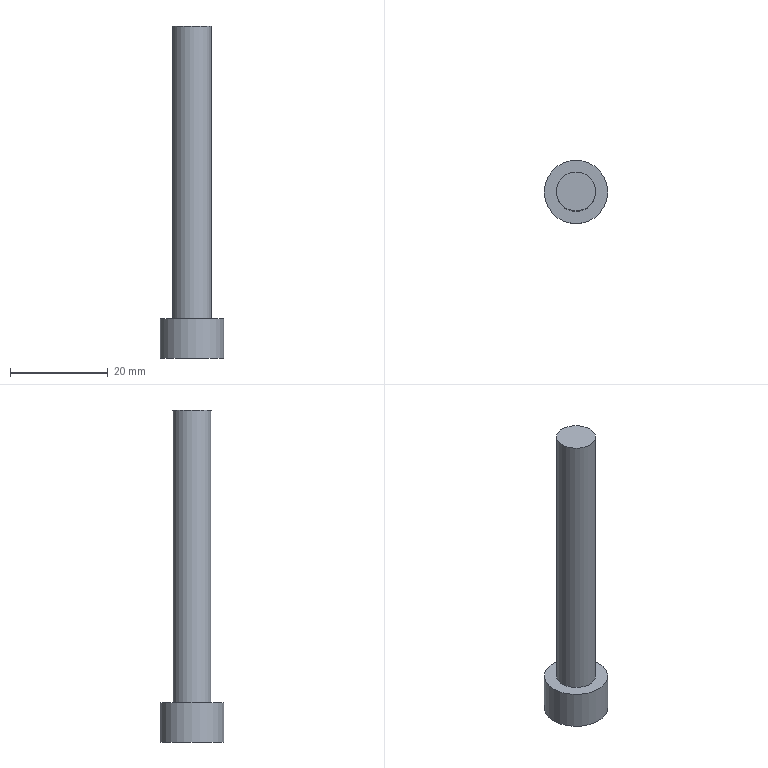Part | STEP file | 1 solid | 12 faces | box 13 x 13 x 68 mm | volume 3913 mm3 | plane 10 | cylinder 2 | commonest cylinder face diameters 8 x1 13 x1
STEP:
#1=CARTESIAN_POINT('',(0.,0.,0.));
#2=DIRECTION('',(0.,0.,1.));
#3=DIRECTION('',(1.,0.,0.));
#4=AXIS2_PLACEMENT_3D('',#1,#2,#3);
#5=CARTESIAN_POINT('',(1550.747,352.48,-93.381));
#6=VERTEX_POINT('',#5);
#7=CARTESIAN_POINT('',(1557.247,352.48,-93.381));
#8=DIRECTION('',(0.,0.,-1.));
#9=DIRECTION('',(-1.,0.,0.));
#10=AXIS2_PLACEMENT_3D('',#7,#8,#9);
#11=CIRCLE('',#10,6.5);
#12=CARTESIAN_POINT('',(1550.747,352.48,-93.381));
#13=DIRECTION('',(0.,0.,1.));
#14=DIRECTION('',(1.,0.,0.));
#15=AXIS2_PLACEMENT_3D('',#12,#13,#14);
#16=PLANE('',#15);
#17=CARTESIAN_POINT('',(0.,0.));
#18=CARTESIAN_POINT('',(0.,11.258));
#19=CARTESIAN_POINT('',(9.75,5.629));
#20=CARTESIAN_POINT('',(19.5,0.));
#21=CARTESIAN_POINT('',(9.75,-5.629));
#22=CARTESIAN_POINT('',(0.,-11.258));
#23=CARTESIAN_POINT('',(0.,0.));
#24=(BOUNDED_CURVE()B_SPLINE_CURVE(2,(#17,#18,#19,#20,#21,#22,#23),.UNSPECIFIED.,.T.,.F.)B_SPLINE_CURVE_WITH_KNOTS((1,2,2,2,2,1),(-2.094,0.,2.094,4.189,6.283,8.378),.UNSPECIFIED.)CURVE()GEOMETRIC_REPRESENTATION_ITEM()RATIONAL_B_SPLINE_CURVE((1.,0.5,1.,0.5,1.,0.5,1.))REPRESENTATION_ITEM(''));
#25=(GEOMETRIC_REPRESENTATION_CONTEXT(2)PARAMETRIC_REPRESENTATION_CONTEXT()REPRESENTATION_CONTEXT('',''));
#26=DEFINITIONAL_REPRESENTATION('',(#24),#25);
#27=PCURVE('',#16,#26);
#28=CARTESIAN_POINT('',(1557.247,352.48,-38.481));
#29=DIRECTION('',(0.,0.,-1.));
#30=DIRECTION('',(-1.,0.,0.));
#31=AXIS2_PLACEMENT_3D('',#28,#29,#30);
#32=CYLINDRICAL_SURFACE('',#31,6.5);
#33=CARTESIAN_POINT('',(0.,54.9));
#34=DIRECTION('',(1.,0.));
#35=VECTOR('',#34,1.);
#36=LINE('',#33,#35);
#37=(GEOMETRIC_REPRESENTATION_CONTEXT(2)PARAMETRIC_REPRESENTATION_CONTEXT()REPRESENTATION_CONTEXT('',''));
#38=DEFINITIONAL_REPRESENTATION('',(#36),#37);
#39=PCURVE('',#32,#38);
#40=SURFACE_CURVE('',#11,(#27,#39),.PCURVE_S1.);
#41=EDGE_CURVE('',#6,#6,#40,.T.);
#42=ORIENTED_EDGE('',*,*,#41,.T.);
#43=EDGE_LOOP('',(#42));
#44=FACE_BOUND('',#43,.T.);
#45=CARTESIAN_POINT('',(1558.979,355.48,-93.381));
#46=VERTEX_POINT('',#45);
#47=CARTESIAN_POINT('',(1555.515,355.48,-93.381));
#48=VERTEX_POINT('',#47);
#49=CARTESIAN_POINT('',(1558.979,355.48,-93.381));
#50=DIRECTION('',(-1.,0.,0.));
#51=VECTOR('',#50,1.);
#52=LINE('',#49,#51);
#53=CARTESIAN_POINT('',(8.232,3.));
#54=DIRECTION('',(-1.,0.));
#55=VECTOR('',#54,1.);
#56=LINE('',#53,#55);
#57=(GEOMETRIC_REPRESENTATION_CONTEXT(2)PARAMETRIC_REPRESENTATION_CONTEXT()REPRESENTATION_CONTEXT('',''));
#58=DEFINITIONAL_REPRESENTATION('',(#56),#57);
#59=PCURVE('',#16,#58);
#60=CARTESIAN_POINT('',(1558.979,355.48,-88.101));
#61=DIRECTION('',(0.,-1.,0.));
#62=DIRECTION('',(-1.,0.,0.));
#63=AXIS2_PLACEMENT_3D('',#60,#61,#62);
#64=PLANE('',#63);
#65=CARTESIAN_POINT('',(0.,5.28));
#66=DIRECTION('',(1.,0.));
#67=VECTOR('',#66,1.);
#68=LINE('',#65,#67);
#69=(GEOMETRIC_REPRESENTATION_CONTEXT(2)PARAMETRIC_REPRESENTATION_CONTEXT()REPRESENTATION_CONTEXT('',''));
#70=DEFINITIONAL_REPRESENTATION('',(#68),#69);
#71=PCURVE('',#64,#70);
#72=SURFACE_CURVE('',#52,(#59,#71),.PCURVE_S1.);
#73=EDGE_CURVE('',#46,#48,#72,.T.);
#74=ORIENTED_EDGE('',*,*,#73,.T.);
#75=CARTESIAN_POINT('',(1553.783,352.48,-93.381));
#76=VERTEX_POINT('',#75);
#77=CARTESIAN_POINT('',(1555.515,355.48,-93.381));
#78=DIRECTION('',(-0.5,-0.866,0.));
#79=VECTOR('',#78,1.);
#80=LINE('',#77,#79);
#81=CARTESIAN_POINT('',(4.768,3.));
#82=DIRECTION('',(-0.5,-0.866));
#83=VECTOR('',#82,1.);
#84=LINE('',#81,#83);
#85=(GEOMETRIC_REPRESENTATION_CONTEXT(2)PARAMETRIC_REPRESENTATION_CONTEXT()REPRESENTATION_CONTEXT('',''));
#86=DEFINITIONAL_REPRESENTATION('',(#84),#85);
#87=PCURVE('',#16,#86);
#88=CARTESIAN_POINT('',(1555.515,355.48,-88.101));
#89=DIRECTION('',(0.866,-0.5,0.));
#90=DIRECTION('',(-0.5,-0.866,0.));
#91=AXIS2_PLACEMENT_3D('',#88,#89,#90);
#92=PLANE('',#91);
#93=CARTESIAN_POINT('',(0.,5.28));
#94=DIRECTION('',(1.,0.));
#95=VECTOR('',#94,1.);
#96=LINE('',#93,#95);
#97=(GEOMETRIC_REPRESENTATION_CONTEXT(2)PARAMETRIC_REPRESENTATION_CONTEXT()REPRESENTATION_CONTEXT('',''));
#98=DEFINITIONAL_REPRESENTATION('',(#96),#97);
#99=PCURVE('',#92,#98);
#100=SURFACE_CURVE('',#80,(#87,#99),.PCURVE_S1.);
#101=EDGE_CURVE('',#48,#76,#100,.T.);
#102=ORIENTED_EDGE('',*,*,#101,.T.);
#103=CARTESIAN_POINT('',(1555.515,349.48,-93.381));
#104=VERTEX_POINT('',#103);
#105=CARTESIAN_POINT('',(1553.783,352.48,-93.381));
#106=DIRECTION('',(0.5,-0.866,0.));
#107=VECTOR('',#106,1.);
#108=LINE('',#105,#107);
#109=CARTESIAN_POINT('',(3.036,0.));
#110=DIRECTION('',(0.5,-0.866));
#111=VECTOR('',#110,1.);
#112=LINE('',#109,#111);
#113=(GEOMETRIC_REPRESENTATION_CONTEXT(2)PARAMETRIC_REPRESENTATION_CONTEXT()REPRESENTATION_CONTEXT('',''));
#114=DEFINITIONAL_REPRESENTATION('',(#112),#113);
#115=PCURVE('',#16,#114);
#116=CARTESIAN_POINT('',(1553.783,352.48,-88.101));
#117=DIRECTION('',(0.866,0.5,0.));
#118=DIRECTION('',(0.5,-0.866,0.));
#119=AXIS2_PLACEMENT_3D('',#116,#117,#118);
#120=PLANE('',#119);
#121=CARTESIAN_POINT('',(0.,5.28));
#122=DIRECTION('',(1.,0.));
#123=VECTOR('',#122,1.);
#124=LINE('',#121,#123);
#125=(GEOMETRIC_REPRESENTATION_CONTEXT(2)PARAMETRIC_REPRESENTATION_CONTEXT()REPRESENTATION_CONTEXT('',''));
#126=DEFINITIONAL_REPRESENTATION('',(#124),#125);
#127=PCURVE('',#120,#126);
#128=SURFACE_CURVE('',#108,(#115,#127),.PCURVE_S1.);
#129=EDGE_CURVE('',#76,#104,#128,.T.);
#130=ORIENTED_EDGE('',*,*,#129,.T.);
#131=CARTESIAN_POINT('',(1558.979,349.48,-93.381));
#132=VERTEX_POINT('',#131);
#133=CARTESIAN_POINT('',(1555.515,349.48,-93.381));
#134=DIRECTION('',(1.,0.,0.));
#135=VECTOR('',#134,1.);
#136=LINE('',#133,#135);
#137=CARTESIAN_POINT('',(4.768,-3.));
#138=DIRECTION('',(1.,0.));
#139=VECTOR('',#138,1.);
#140=LINE('',#137,#139);
#141=(GEOMETRIC_REPRESENTATION_CONTEXT(2)PARAMETRIC_REPRESENTATION_CONTEXT()REPRESENTATION_CONTEXT('',''));
#142=DEFINITIONAL_REPRESENTATION('',(#140),#141);
#143=PCURVE('',#16,#142);
#144=CARTESIAN_POINT('',(1555.515,349.48,-88.101));
#145=DIRECTION('',(0.,1.,0.));
#146=DIRECTION('',(1.,0.,0.));
#147=AXIS2_PLACEMENT_3D('',#144,#145,#146);
#148=PLANE('',#147);
#149=CARTESIAN_POINT('',(0.,5.28));
#150=DIRECTION('',(1.,0.));
#151=VECTOR('',#150,1.);
#152=LINE('',#149,#151);
#153=(GEOMETRIC_REPRESENTATION_CONTEXT(2)PARAMETRIC_REPRESENTATION_CONTEXT()REPRESENTATION_CONTEXT('',''));
#154=DEFINITIONAL_REPRESENTATION('',(#152),#153);
#155=PCURVE('',#148,#154);
#156=SURFACE_CURVE('',#136,(#143,#155),.PCURVE_S1.);
#157=EDGE_CURVE('',#104,#132,#156,.T.);
#158=ORIENTED_EDGE('',*,*,#157,.T.);
#159=CARTESIAN_POINT('',(1560.711,352.48,-93.381));
#160=VERTEX_POINT('',#159);
#161=CARTESIAN_POINT('',(1558.979,349.48,-93.381));
#162=DIRECTION('',(0.5,0.866,0.));
#163=VECTOR('',#162,1.);
#164=LINE('',#161,#163);
#165=CARTESIAN_POINT('',(8.232,-3.));
#166=DIRECTION('',(0.5,0.866));
#167=VECTOR('',#166,1.);
#168=LINE('',#165,#167);
#169=(GEOMETRIC_REPRESENTATION_CONTEXT(2)PARAMETRIC_REPRESENTATION_CONTEXT()REPRESENTATION_CONTEXT('',''));
#170=DEFINITIONAL_REPRESENTATION('',(#168),#169);
#171=PCURVE('',#16,#170);
#172=CARTESIAN_POINT('',(1558.979,349.48,-88.101));
#173=DIRECTION('',(-0.866,0.5,0.));
#174=DIRECTION('',(0.5,0.866,0.));
#175=AXIS2_PLACEMENT_3D('',#172,#173,#174);
#176=PLANE('',#175);
#177=CARTESIAN_POINT('',(0.,5.28));
#178=DIRECTION('',(1.,0.));
#179=VECTOR('',#178,1.);
#180=LINE('',#177,#179);
#181=(GEOMETRIC_REPRESENTATION_CONTEXT(2)PARAMETRIC_REPRESENTATION_CONTEXT()REPRESENTATION_CONTEXT('',''));
#182=DEFINITIONAL_REPRESENTATION('',(#180),#181);
#183=PCURVE('',#176,#182);
#184=SURFACE_CURVE('',#164,(#171,#183),.PCURVE_S1.);
#185=EDGE_CURVE('',#132,#160,#184,.T.);
#186=ORIENTED_EDGE('',*,*,#185,.T.);
#187=CARTESIAN_POINT('',(1560.711,352.48,-93.381));
#188=DIRECTION('',(-0.5,0.866,0.));
#189=VECTOR('',#188,1.);
#190=LINE('',#187,#189);
#191=CARTESIAN_POINT('',(9.964,0.));
#192=DIRECTION('',(-0.5,0.866));
#193=VECTOR('',#192,1.);
#194=LINE('',#191,#193);
#195=(GEOMETRIC_REPRESENTATION_CONTEXT(2)PARAMETRIC_REPRESENTATION_CONTEXT()REPRESENTATION_CONTEXT('',''));
#196=DEFINITIONAL_REPRESENTATION('',(#194),#195);
#197=PCURVE('',#16,#196);
#198=CARTESIAN_POINT('',(1560.711,352.48,-88.101));
#199=DIRECTION('',(-0.866,-0.5,0.));
#200=DIRECTION('',(-0.5,0.866,0.));
#201=AXIS2_PLACEMENT_3D('',#198,#199,#200);
#202=PLANE('',#201);
#203=CARTESIAN_POINT('',(0.,5.28));
#204=DIRECTION('',(1.,0.));
#205=VECTOR('',#204,1.);
#206=LINE('',#203,#205);
#207=(GEOMETRIC_REPRESENTATION_CONTEXT(2)PARAMETRIC_REPRESENTATION_CONTEXT()REPRESENTATION_CONTEXT('',''));
#208=DEFINITIONAL_REPRESENTATION('',(#206),#207);
#209=PCURVE('',#202,#208);
#210=SURFACE_CURVE('',#190,(#197,#209),.PCURVE_S1.);
#211=EDGE_CURVE('',#160,#46,#210,.T.);
#212=ORIENTED_EDGE('',*,*,#211,.T.);
#213=EDGE_LOOP('',(#74,#102,#130,#158,#186,#212));
#214=FACE_BOUND('',#213,.T.);
#215=ADVANCED_FACE('',(#44,#214),#16,.F.);
#216=ORIENTED_EDGE('',*,*,#41,.F.);
#217=CARTESIAN_POINT('',(1550.747,352.48,-85.381));
#218=VERTEX_POINT('',#217);
#219=CARTESIAN_POINT('',(1550.747,352.48,-85.381));
#220=CARTESIAN_POINT('',(1550.747,352.48,-93.381));
#221=B_SPLINE_CURVE_WITH_KNOTS('',1,(#219,#220),.UNSPECIFIED.,.F.,.F.,(2,2),(46.9,54.9),.PIECEWISE_BEZIER_KNOTS.);
#222=CARTESIAN_POINT('',(0.,0.));
#223=DIRECTION('',(0.,1.));
#224=VECTOR('',#223,1.);
#225=LINE('',#222,#224);
#226=(GEOMETRIC_REPRESENTATION_CONTEXT(2)PARAMETRIC_REPRESENTATION_CONTEXT()REPRESENTATION_CONTEXT('',''));
#227=DEFINITIONAL_REPRESENTATION('',(#225),#226);
#228=PCURVE('',#32,#227);
#229=CARTESIAN_POINT('',(6.283,0.));
#230=DIRECTION('',(0.,1.));
#231=VECTOR('',#230,1.);
#232=LINE('',#229,#231);
#233=(GEOMETRIC_REPRESENTATION_CONTEXT(2)PARAMETRIC_REPRESENTATION_CONTEXT()REPRESENTATION_CONTEXT('',''));
#234=DEFINITIONAL_REPRESENTATION('',(#232),#233);
#235=PCURVE('',#32,#234);
#236=SEAM_CURVE('',#221,(#228,#235),.PCURVE_S1.);
#237=EDGE_CURVE('',#218,#6,#236,.T.);
#238=ORIENTED_EDGE('',*,*,#237,.F.);
#239=CARTESIAN_POINT('',(1557.247,352.48,-85.381));
#240=DIRECTION('',(0.,0.,-1.));
#241=DIRECTION('',(-1.,0.,0.));
#242=AXIS2_PLACEMENT_3D('',#239,#240,#241);
#243=CIRCLE('',#242,6.5);
#244=CARTESIAN_POINT('',(0.,46.9));
#245=DIRECTION('',(1.,0.));
#246=VECTOR('',#245,1.);
#247=LINE('',#244,#246);
#248=(GEOMETRIC_REPRESENTATION_CONTEXT(2)PARAMETRIC_REPRESENTATION_CONTEXT()REPRESENTATION_CONTEXT('',''));
#249=DEFINITIONAL_REPRESENTATION('',(#247),#248);
#250=PCURVE('',#32,#249);
#251=CARTESIAN_POINT('',(1553.247,352.48,-85.381));
#252=DIRECTION('',(0.,0.,-1.));
#253=DIRECTION('',(-1.,0.,0.));
#254=AXIS2_PLACEMENT_3D('',#251,#252,#253);
#255=PLANE('',#254);
#256=CARTESIAN_POINT('',(-4.,0.));
#257=DIRECTION('',(1.,0.));
#258=AXIS2_PLACEMENT_2D('',#256,#257);
#259=CIRCLE('',#258,6.5);
#260=(GEOMETRIC_REPRESENTATION_CONTEXT(2)PARAMETRIC_REPRESENTATION_CONTEXT()REPRESENTATION_CONTEXT('',''));
#261=DEFINITIONAL_REPRESENTATION('',(#259),#260);
#262=PCURVE('',#255,#261);
#263=SURFACE_CURVE('',#243,(#250,#262),.PCURVE_S1.);
#264=EDGE_CURVE('',#218,#218,#263,.T.);
#265=ORIENTED_EDGE('',*,*,#264,.T.);
#266=ORIENTED_EDGE('',*,*,#237,.T.);
#267=EDGE_LOOP('',(#216,#238,#265,#266));
#268=FACE_BOUND('',#267,.T.);
#269=ADVANCED_FACE('',(#268),#32,.T.);
#270=ORIENTED_EDGE('',*,*,#264,.F.);
#271=EDGE_LOOP('',(#270));
#272=FACE_BOUND('',#271,.T.);
#273=CARTESIAN_POINT('',(1553.247,352.48,-85.381));
#274=VERTEX_POINT('',#273);
#275=CARTESIAN_POINT('',(1557.247,352.48,-85.381));
#276=DIRECTION('',(0.,0.,-1.));
#277=DIRECTION('',(-1.,0.,0.));
#278=AXIS2_PLACEMENT_3D('',#275,#276,#277);
#279=CIRCLE('',#278,4.);
#280=CARTESIAN_POINT('',(-4.,0.));
#281=DIRECTION('',(1.,0.));
#282=AXIS2_PLACEMENT_2D('',#280,#281);
#283=CIRCLE('',#282,4.);
#284=(GEOMETRIC_REPRESENTATION_CONTEXT(2)PARAMETRIC_REPRESENTATION_CONTEXT()REPRESENTATION_CONTEXT('',''));
#285=DEFINITIONAL_REPRESENTATION('',(#283),#284);
#286=PCURVE('',#255,#285);
#287=CARTESIAN_POINT('',(1557.247,352.48,-38.481));
#288=DIRECTION('',(0.,0.,-1.));
#289=DIRECTION('',(-1.,0.,0.));
#290=AXIS2_PLACEMENT_3D('',#287,#288,#289);
#291=CYLINDRICAL_SURFACE('',#290,4.);
#292=CARTESIAN_POINT('',(0.,46.9));
#293=DIRECTION('',(1.,0.));
#294=VECTOR('',#293,1.);
#295=LINE('',#292,#294);
#296=(GEOMETRIC_REPRESENTATION_CONTEXT(2)PARAMETRIC_REPRESENTATION_CONTEXT()REPRESENTATION_CONTEXT('',''));
#297=DEFINITIONAL_REPRESENTATION('',(#295),#296);
#298=PCURVE('',#291,#297);
#299=SURFACE_CURVE('',#279,(#286,#298),.PCURVE_S1.);
#300=EDGE_CURVE('',#274,#274,#299,.T.);
#301=ORIENTED_EDGE('',*,*,#300,.T.);
#302=EDGE_LOOP('',(#301));
#303=FACE_BOUND('',#302,.T.);
#304=ADVANCED_FACE('',(#272,#303),#255,.F.);
#305=ORIENTED_EDGE('',*,*,#300,.F.);
#306=CARTESIAN_POINT('',(1553.247,352.48,-25.381));
#307=VERTEX_POINT('',#306);
#308=CARTESIAN_POINT('',(1553.247,352.48,-25.381));
#309=CARTESIAN_POINT('',(1553.247,352.48,-85.381));
#310=B_SPLINE_CURVE_WITH_KNOTS('',1,(#308,#309),.UNSPECIFIED.,.F.,.F.,(2,2),(-13.1,46.9),.PIECEWISE_BEZIER_KNOTS.);
#311=CARTESIAN_POINT('',(0.,0.));
#312=DIRECTION('',(0.,1.));
#313=VECTOR('',#312,1.);
#314=LINE('',#311,#313);
#315=(GEOMETRIC_REPRESENTATION_CONTEXT(2)PARAMETRIC_REPRESENTATION_CONTEXT()REPRESENTATION_CONTEXT('',''));
#316=DEFINITIONAL_REPRESENTATION('',(#314),#315);
#317=PCURVE('',#291,#316);
#318=CARTESIAN_POINT('',(6.283,0.));
#319=DIRECTION('',(0.,1.));
#320=VECTOR('',#319,1.);
#321=LINE('',#318,#320);
#322=(GEOMETRIC_REPRESENTATION_CONTEXT(2)PARAMETRIC_REPRESENTATION_CONTEXT()REPRESENTATION_CONTEXT('',''));
#323=DEFINITIONAL_REPRESENTATION('',(#321),#322);
#324=PCURVE('',#291,#323);
#325=SEAM_CURVE('',#310,(#317,#324),.PCURVE_S1.);
#326=EDGE_CURVE('',#307,#274,#325,.T.);
#327=ORIENTED_EDGE('',*,*,#326,.F.);
#328=CARTESIAN_POINT('',(1557.247,352.48,-25.381));
#329=DIRECTION('',(0.,0.,-1.));
#330=DIRECTION('',(-1.,0.,0.));
#331=AXIS2_PLACEMENT_3D('',#328,#329,#330);
#332=CIRCLE('',#331,4.);
#333=CARTESIAN_POINT('',(0.,-13.1));
#334=DIRECTION('',(1.,0.));
#335=VECTOR('',#334,1.);
#336=LINE('',#333,#335);
#337=(GEOMETRIC_REPRESENTATION_CONTEXT(2)PARAMETRIC_REPRESENTATION_CONTEXT()REPRESENTATION_CONTEXT('',''));
#338=DEFINITIONAL_REPRESENTATION('',(#336),#337);
#339=PCURVE('',#291,#338);
#340=CARTESIAN_POINT('',(1557.247,352.48,-25.381));
#341=DIRECTION('',(0.,0.,-1.));
#342=DIRECTION('',(-1.,0.,0.));
#343=AXIS2_PLACEMENT_3D('',#340,#341,#342);
#344=PLANE('',#343);
#345=CARTESIAN_POINT('',(0.,0.));
#346=DIRECTION('',(1.,0.));
#347=AXIS2_PLACEMENT_2D('',#345,#346);
#348=CIRCLE('',#347,4.);
#349=(GEOMETRIC_REPRESENTATION_CONTEXT(2)PARAMETRIC_REPRESENTATION_CONTEXT()REPRESENTATION_CONTEXT('',''));
#350=DEFINITIONAL_REPRESENTATION('',(#348),#349);
#351=PCURVE('',#344,#350);
#352=SURFACE_CURVE('',#332,(#339,#351),.PCURVE_S1.);
#353=EDGE_CURVE('',#307,#307,#352,.T.);
#354=ORIENTED_EDGE('',*,*,#353,.T.);
#355=ORIENTED_EDGE('',*,*,#326,.T.);
#356=EDGE_LOOP('',(#305,#327,#354,#355));
#357=FACE_BOUND('',#356,.T.);
#358=ADVANCED_FACE('',(#357),#291,.T.);
#359=ORIENTED_EDGE('',*,*,#353,.F.);
#360=EDGE_LOOP('',(#359));
#361=FACE_BOUND('',#360,.T.);
#362=ADVANCED_FACE('',(#361),#344,.F.);
#363=ORIENTED_EDGE('',*,*,#73,.F.);
#364=CARTESIAN_POINT('',(1558.979,355.48,-88.101));
#365=VERTEX_POINT('',#364);
#366=CARTESIAN_POINT('',(1558.979,355.48,-88.101));
#367=DIRECTION('',(0.,0.,1.));
#368=VECTOR('',#367,1.);
#369=LINE('',#366,#368);
#370=CARTESIAN_POINT('',(0.,0.));
#371=DIRECTION('',(0.,-1.));
#372=VECTOR('',#371,1.);
#373=LINE('',#370,#372);
#374=(GEOMETRIC_REPRESENTATION_CONTEXT(2)PARAMETRIC_REPRESENTATION_CONTEXT()REPRESENTATION_CONTEXT('',''));
#375=DEFINITIONAL_REPRESENTATION('',(#373),#374);
#376=PCURVE('',#64,#375);
#377=CARTESIAN_POINT('',(3.464,0.));
#378=DIRECTION('',(0.,-1.));
#379=VECTOR('',#378,1.);
#380=LINE('',#377,#379);
#381=(GEOMETRIC_REPRESENTATION_CONTEXT(2)PARAMETRIC_REPRESENTATION_CONTEXT()REPRESENTATION_CONTEXT('',''));
#382=DEFINITIONAL_REPRESENTATION('',(#380),#381);
#383=PCURVE('',#202,#382);
#384=SURFACE_CURVE('',#369,(#376,#383),.PCURVE_S1.);
#385=EDGE_CURVE('',#46,#365,#384,.T.);
#386=ORIENTED_EDGE('',*,*,#385,.T.);
#387=CARTESIAN_POINT('',(1555.515,355.48,-88.101));
#388=VERTEX_POINT('',#387);
#389=CARTESIAN_POINT('',(1558.979,355.48,-88.101));
#390=DIRECTION('',(1.,0.,0.));
#391=VECTOR('',#390,1.);
#392=LINE('',#389,#391);
#393=CARTESIAN_POINT('',(0.,0.));
#394=DIRECTION('',(-1.,0.));
#395=VECTOR('',#394,1.);
#396=LINE('',#393,#395);
#397=(GEOMETRIC_REPRESENTATION_CONTEXT(2)PARAMETRIC_REPRESENTATION_CONTEXT()REPRESENTATION_CONTEXT('',''));
#398=DEFINITIONAL_REPRESENTATION('',(#396),#397);
#399=PCURVE('',#64,#398);
#400=CARTESIAN_POINT('',(1557.247,352.48,-88.101));
#401=DIRECTION('',(0.,0.,1.));
#402=DIRECTION('',(1.,0.,0.));
#403=AXIS2_PLACEMENT_3D('',#400,#401,#402);
#404=PLANE('',#403);
#405=CARTESIAN_POINT('',(1.732,3.));
#406=DIRECTION('',(1.,0.));
#407=VECTOR('',#406,1.);
#408=LINE('',#405,#407);
#409=(GEOMETRIC_REPRESENTATION_CONTEXT(2)PARAMETRIC_REPRESENTATION_CONTEXT()REPRESENTATION_CONTEXT('',''));
#410=DEFINITIONAL_REPRESENTATION('',(#408),#409);
#411=PCURVE('',#404,#410);
#412=SURFACE_CURVE('',#392,(#399,#411),.PCURVE_S1.);
#413=EDGE_CURVE('',#388,#365,#412,.T.);
#414=ORIENTED_EDGE('',*,*,#413,.F.);
#415=CARTESIAN_POINT('',(1555.515,355.48,-88.101));
#416=DIRECTION('',(0.,0.,1.));
#417=VECTOR('',#416,1.);
#418=LINE('',#415,#417);
#419=CARTESIAN_POINT('',(3.464,0.));
#420=DIRECTION('',(0.,-1.));
#421=VECTOR('',#420,1.);
#422=LINE('',#419,#421);
#423=(GEOMETRIC_REPRESENTATION_CONTEXT(2)PARAMETRIC_REPRESENTATION_CONTEXT()REPRESENTATION_CONTEXT('',''));
#424=DEFINITIONAL_REPRESENTATION('',(#422),#423);
#425=PCURVE('',#64,#424);
#426=CARTESIAN_POINT('',(0.,0.));
#427=DIRECTION('',(0.,-1.));
#428=VECTOR('',#427,1.);
#429=LINE('',#426,#428);
#430=(GEOMETRIC_REPRESENTATION_CONTEXT(2)PARAMETRIC_REPRESENTATION_CONTEXT()REPRESENTATION_CONTEXT('',''));
#431=DEFINITIONAL_REPRESENTATION('',(#429),#430);
#432=PCURVE('',#92,#431);
#433=SURFACE_CURVE('',#418,(#425,#432),.PCURVE_S1.);
#434=EDGE_CURVE('',#48,#388,#433,.T.);
#435=ORIENTED_EDGE('',*,*,#434,.F.);
#436=EDGE_LOOP('',(#363,#386,#414,#435));
#437=FACE_BOUND('',#436,.T.);
#438=ADVANCED_FACE('',(#437),#64,.T.);
#439=ORIENTED_EDGE('',*,*,#101,.F.);
#440=ORIENTED_EDGE('',*,*,#434,.T.);
#441=CARTESIAN_POINT('',(1553.783,352.48,-88.101));
#442=VERTEX_POINT('',#441);
#443=CARTESIAN_POINT('',(1555.515,355.48,-88.101));
#444=DIRECTION('',(0.5,0.866,0.));
#445=VECTOR('',#444,1.);
#446=LINE('',#443,#445);
#447=CARTESIAN_POINT('',(0.,0.));
#448=DIRECTION('',(-1.,0.));
#449=VECTOR('',#448,1.);
#450=LINE('',#447,#449);
#451=(GEOMETRIC_REPRESENTATION_CONTEXT(2)PARAMETRIC_REPRESENTATION_CONTEXT()REPRESENTATION_CONTEXT('',''));
#452=DEFINITIONAL_REPRESENTATION('',(#450),#451);
#453=PCURVE('',#92,#452);
#454=CARTESIAN_POINT('',(-1.732,3.));
#455=DIRECTION('',(0.5,0.866));
#456=VECTOR('',#455,1.);
#457=LINE('',#454,#456);
#458=(GEOMETRIC_REPRESENTATION_CONTEXT(2)PARAMETRIC_REPRESENTATION_CONTEXT()REPRESENTATION_CONTEXT('',''));
#459=DEFINITIONAL_REPRESENTATION('',(#457),#458);
#460=PCURVE('',#404,#459);
#461=SURFACE_CURVE('',#446,(#453,#460),.PCURVE_S1.);
#462=EDGE_CURVE('',#442,#388,#461,.T.);
#463=ORIENTED_EDGE('',*,*,#462,.F.);
#464=CARTESIAN_POINT('',(1553.783,352.48,-88.101));
#465=DIRECTION('',(0.,0.,1.));
#466=VECTOR('',#465,1.);
#467=LINE('',#464,#466);
#468=CARTESIAN_POINT('',(3.464,0.));
#469=DIRECTION('',(0.,-1.));
#470=VECTOR('',#469,1.);
#471=LINE('',#468,#470);
#472=(GEOMETRIC_REPRESENTATION_CONTEXT(2)PARAMETRIC_REPRESENTATION_CONTEXT()REPRESENTATION_CONTEXT('',''));
#473=DEFINITIONAL_REPRESENTATION('',(#471),#472);
#474=PCURVE('',#92,#473);
#475=CARTESIAN_POINT('',(0.,0.));
#476=DIRECTION('',(0.,-1.));
#477=VECTOR('',#476,1.);
#478=LINE('',#475,#477);
#479=(GEOMETRIC_REPRESENTATION_CONTEXT(2)PARAMETRIC_REPRESENTATION_CONTEXT()REPRESENTATION_CONTEXT('',''));
#480=DEFINITIONAL_REPRESENTATION('',(#478),#479);
#481=PCURVE('',#120,#480);
#482=SURFACE_CURVE('',#467,(#474,#481),.PCURVE_S1.);
#483=EDGE_CURVE('',#76,#442,#482,.T.);
#484=ORIENTED_EDGE('',*,*,#483,.F.);
#485=EDGE_LOOP('',(#439,#440,#463,#484));
#486=FACE_BOUND('',#485,.T.);
#487=ADVANCED_FACE('',(#486),#92,.T.);
#488=ORIENTED_EDGE('',*,*,#129,.F.);
#489=ORIENTED_EDGE('',*,*,#483,.T.);
#490=CARTESIAN_POINT('',(1555.515,349.48,-88.101));
#491=VERTEX_POINT('',#490);
#492=CARTESIAN_POINT('',(1553.783,352.48,-88.101));
#493=DIRECTION('',(-0.5,0.866,0.));
#494=VECTOR('',#493,1.);
#495=LINE('',#492,#494);
#496=CARTESIAN_POINT('',(0.,0.));
#497=DIRECTION('',(-1.,0.));
#498=VECTOR('',#497,1.);
#499=LINE('',#496,#498);
#500=(GEOMETRIC_REPRESENTATION_CONTEXT(2)PARAMETRIC_REPRESENTATION_CONTEXT()REPRESENTATION_CONTEXT('',''));
#501=DEFINITIONAL_REPRESENTATION('',(#499),#500);
#502=PCURVE('',#120,#501);
#503=CARTESIAN_POINT('',(-3.464,0.));
#504=DIRECTION('',(-0.5,0.866));
#505=VECTOR('',#504,1.);
#506=LINE('',#503,#505);
#507=(GEOMETRIC_REPRESENTATION_CONTEXT(2)PARAMETRIC_REPRESENTATION_CONTEXT()REPRESENTATION_CONTEXT('',''));
#508=DEFINITIONAL_REPRESENTATION('',(#506),#507);
#509=PCURVE('',#404,#508);
#510=SURFACE_CURVE('',#495,(#502,#509),.PCURVE_S1.);
#511=EDGE_CURVE('',#491,#442,#510,.T.);
#512=ORIENTED_EDGE('',*,*,#511,.F.);
#513=CARTESIAN_POINT('',(1555.515,349.48,-88.101));
#514=DIRECTION('',(0.,0.,1.));
#515=VECTOR('',#514,1.);
#516=LINE('',#513,#515);
#517=CARTESIAN_POINT('',(3.464,0.));
#518=DIRECTION('',(0.,-1.));
#519=VECTOR('',#518,1.);
#520=LINE('',#517,#519);
#521=(GEOMETRIC_REPRESENTATION_CONTEXT(2)PARAMETRIC_REPRESENTATION_CONTEXT()REPRESENTATION_CONTEXT('',''));
#522=DEFINITIONAL_REPRESENTATION('',(#520),#521);
#523=PCURVE('',#120,#522);
#524=CARTESIAN_POINT('',(0.,0.));
#525=DIRECTION('',(0.,-1.));
#526=VECTOR('',#525,1.);
#527=LINE('',#524,#526);
#528=(GEOMETRIC_REPRESENTATION_CONTEXT(2)PARAMETRIC_REPRESENTATION_CONTEXT()REPRESENTATION_CONTEXT('',''));
#529=DEFINITIONAL_REPRESENTATION('',(#527),#528);
#530=PCURVE('',#148,#529);
#531=SURFACE_CURVE('',#516,(#523,#530),.PCURVE_S1.);
#532=EDGE_CURVE('',#104,#491,#531,.T.);
#533=ORIENTED_EDGE('',*,*,#532,.F.);
#534=EDGE_LOOP('',(#488,#489,#512,#533));
#535=FACE_BOUND('',#534,.T.);
#536=ADVANCED_FACE('',(#535),#120,.T.);
#537=ORIENTED_EDGE('',*,*,#157,.F.);
#538=ORIENTED_EDGE('',*,*,#532,.T.);
#539=CARTESIAN_POINT('',(1558.979,349.48,-88.101));
#540=VERTEX_POINT('',#539);
#541=CARTESIAN_POINT('',(1555.515,349.48,-88.101));
#542=DIRECTION('',(-1.,0.,0.));
#543=VECTOR('',#542,1.);
#544=LINE('',#541,#543);
#545=CARTESIAN_POINT('',(0.,0.));
#546=DIRECTION('',(-1.,0.));
#547=VECTOR('',#546,1.);
#548=LINE('',#545,#547);
#549=(GEOMETRIC_REPRESENTATION_CONTEXT(2)PARAMETRIC_REPRESENTATION_CONTEXT()REPRESENTATION_CONTEXT('',''));
#550=DEFINITIONAL_REPRESENTATION('',(#548),#549);
#551=PCURVE('',#148,#550);
#552=CARTESIAN_POINT('',(-1.732,-3.));
#553=DIRECTION('',(-1.,0.));
#554=VECTOR('',#553,1.);
#555=LINE('',#552,#554);
#556=(GEOMETRIC_REPRESENTATION_CONTEXT(2)PARAMETRIC_REPRESENTATION_CONTEXT()REPRESENTATION_CONTEXT('',''));
#557=DEFINITIONAL_REPRESENTATION('',(#555),#556);
#558=PCURVE('',#404,#557);
#559=SURFACE_CURVE('',#544,(#551,#558),.PCURVE_S1.);
#560=EDGE_CURVE('',#540,#491,#559,.T.);
#561=ORIENTED_EDGE('',*,*,#560,.F.);
#562=CARTESIAN_POINT('',(1558.979,349.48,-88.101));
#563=DIRECTION('',(0.,0.,1.));
#564=VECTOR('',#563,1.);
#565=LINE('',#562,#564);
#566=CARTESIAN_POINT('',(3.464,0.));
#567=DIRECTION('',(0.,-1.));
#568=VECTOR('',#567,1.);
#569=LINE('',#566,#568);
#570=(GEOMETRIC_REPRESENTATION_CONTEXT(2)PARAMETRIC_REPRESENTATION_CONTEXT()REPRESENTATION_CONTEXT('',''));
#571=DEFINITIONAL_REPRESENTATION('',(#569),#570);
#572=PCURVE('',#148,#571);
#573=CARTESIAN_POINT('',(0.,0.));
#574=DIRECTION('',(0.,-1.));
#575=VECTOR('',#574,1.);
#576=LINE('',#573,#575);
#577=(GEOMETRIC_REPRESENTATION_CONTEXT(2)PARAMETRIC_REPRESENTATION_CONTEXT()REPRESENTATION_CONTEXT('',''));
#578=DEFINITIONAL_REPRESENTATION('',(#576),#577);
#579=PCURVE('',#176,#578);
#580=SURFACE_CURVE('',#565,(#572,#579),.PCURVE_S1.);
#581=EDGE_CURVE('',#132,#540,#580,.T.);
#582=ORIENTED_EDGE('',*,*,#581,.F.);
#583=EDGE_LOOP('',(#537,#538,#561,#582));
#584=FACE_BOUND('',#583,.T.);
#585=ADVANCED_FACE('',(#584),#148,.T.);
#586=ORIENTED_EDGE('',*,*,#185,.F.);
#587=ORIENTED_EDGE('',*,*,#581,.T.);
#588=CARTESIAN_POINT('',(1560.711,352.48,-88.101));
#589=VERTEX_POINT('',#588);
#590=CARTESIAN_POINT('',(1558.979,349.48,-88.101));
#591=DIRECTION('',(-0.5,-0.866,0.));
#592=VECTOR('',#591,1.);
#593=LINE('',#590,#592);
#594=CARTESIAN_POINT('',(0.,0.));
#595=DIRECTION('',(-1.,0.));
#596=VECTOR('',#595,1.);
#597=LINE('',#594,#596);
#598=(GEOMETRIC_REPRESENTATION_CONTEXT(2)PARAMETRIC_REPRESENTATION_CONTEXT()REPRESENTATION_CONTEXT('',''));
#599=DEFINITIONAL_REPRESENTATION('',(#597),#598);
#600=PCURVE('',#176,#599);
#601=CARTESIAN_POINT('',(1.732,-3.));
#602=DIRECTION('',(-0.5,-0.866));
#603=VECTOR('',#602,1.);
#604=LINE('',#601,#603);
#605=(GEOMETRIC_REPRESENTATION_CONTEXT(2)PARAMETRIC_REPRESENTATION_CONTEXT()REPRESENTATION_CONTEXT('',''));
#606=DEFINITIONAL_REPRESENTATION('',(#604),#605);
#607=PCURVE('',#404,#606);
#608=SURFACE_CURVE('',#593,(#600,#607),.PCURVE_S1.);
#609=EDGE_CURVE('',#589,#540,#608,.T.);
#610=ORIENTED_EDGE('',*,*,#609,.F.);
#611=CARTESIAN_POINT('',(1560.711,352.48,-88.101));
#612=DIRECTION('',(0.,0.,1.));
#613=VECTOR('',#612,1.);
#614=LINE('',#611,#613);
#615=CARTESIAN_POINT('',(3.464,0.));
#616=DIRECTION('',(0.,-1.));
#617=VECTOR('',#616,1.);
#618=LINE('',#615,#617);
#619=(GEOMETRIC_REPRESENTATION_CONTEXT(2)PARAMETRIC_REPRESENTATION_CONTEXT()REPRESENTATION_CONTEXT('',''));
#620=DEFINITIONAL_REPRESENTATION('',(#618),#619);
#621=PCURVE('',#176,#620);
#622=CARTESIAN_POINT('',(0.,0.));
#623=DIRECTION('',(0.,-1.));
#624=VECTOR('',#623,1.);
#625=LINE('',#622,#624);
#626=(GEOMETRIC_REPRESENTATION_CONTEXT(2)PARAMETRIC_REPRESENTATION_CONTEXT()REPRESENTATION_CONTEXT('',''));
#627=DEFINITIONAL_REPRESENTATION('',(#625),#626);
#628=PCURVE('',#202,#627);
#629=SURFACE_CURVE('',#614,(#621,#628),.PCURVE_S1.);
#630=EDGE_CURVE('',#160,#589,#629,.T.);
#631=ORIENTED_EDGE('',*,*,#630,.F.);
#632=EDGE_LOOP('',(#586,#587,#610,#631));
#633=FACE_BOUND('',#632,.T.);
#634=ADVANCED_FACE('',(#633),#176,.T.);
#635=ORIENTED_EDGE('',*,*,#211,.F.);
#636=ORIENTED_EDGE('',*,*,#630,.T.);
#637=CARTESIAN_POINT('',(1560.711,352.48,-88.101));
#638=DIRECTION('',(0.5,-0.866,0.));
#639=VECTOR('',#638,1.);
#640=LINE('',#637,#639);
#641=CARTESIAN_POINT('',(0.,0.));
#642=DIRECTION('',(-1.,0.));
#643=VECTOR('',#642,1.);
#644=LINE('',#641,#643);
#645=(GEOMETRIC_REPRESENTATION_CONTEXT(2)PARAMETRIC_REPRESENTATION_CONTEXT()REPRESENTATION_CONTEXT('',''));
#646=DEFINITIONAL_REPRESENTATION('',(#644),#645);
#647=PCURVE('',#202,#646);
#648=CARTESIAN_POINT('',(3.464,0.));
#649=DIRECTION('',(0.5,-0.866));
#650=VECTOR('',#649,1.);
#651=LINE('',#648,#650);
#652=(GEOMETRIC_REPRESENTATION_CONTEXT(2)PARAMETRIC_REPRESENTATION_CONTEXT()REPRESENTATION_CONTEXT('',''));
#653=DEFINITIONAL_REPRESENTATION('',(#651),#652);
#654=PCURVE('',#404,#653);
#655=SURFACE_CURVE('',#640,(#647,#654),.PCURVE_S1.);
#656=EDGE_CURVE('',#365,#589,#655,.T.);
#657=ORIENTED_EDGE('',*,*,#656,.F.);
#658=ORIENTED_EDGE('',*,*,#385,.F.);
#659=EDGE_LOOP('',(#635,#636,#657,#658));
#660=FACE_BOUND('',#659,.T.);
#661=ADVANCED_FACE('',(#660),#202,.T.);
#662=ORIENTED_EDGE('',*,*,#413,.T.);
#663=ORIENTED_EDGE('',*,*,#656,.T.);
#664=ORIENTED_EDGE('',*,*,#609,.T.);
#665=ORIENTED_EDGE('',*,*,#560,.T.);
#666=ORIENTED_EDGE('',*,*,#511,.T.);
#667=ORIENTED_EDGE('',*,*,#462,.T.);
#668=EDGE_LOOP('',(#662,#663,#664,#665,#666,#667));
#669=FACE_BOUND('',#668,.T.);
#670=ADVANCED_FACE('',(#669),#404,.F.);
#671=CLOSED_SHELL('',(#215,#269,#304,#358,#362,#438,#487,#536,#585,#634,#661,#670));
#672=MANIFOLD_SOLID_BREP('',#671);
#673=(LENGTH_UNIT()NAMED_UNIT(*)SI_UNIT(.MILLI.,.METRE.));
#674=UNCERTAINTY_MEASURE_WITH_UNIT(LENGTH_MEASURE(0.000002),#673,'','');
#675=(NAMED_UNIT(*)PLANE_ANGLE_UNIT()SI_UNIT($,.RADIAN.));
#676=(NAMED_UNIT(*)SI_UNIT($,.STERADIAN.)SOLID_ANGLE_UNIT());
#677=(GEOMETRIC_REPRESENTATION_CONTEXT(3)GLOBAL_UNCERTAINTY_ASSIGNED_CONTEXT((#674))GLOBAL_UNIT_ASSIGNED_CONTEXT((#673,#675,#676))REPRESENTATION_CONTEXT('',''));
#678=ADVANCED_BREP_SHAPE_REPRESENTATION('',(#4,#672),#677);